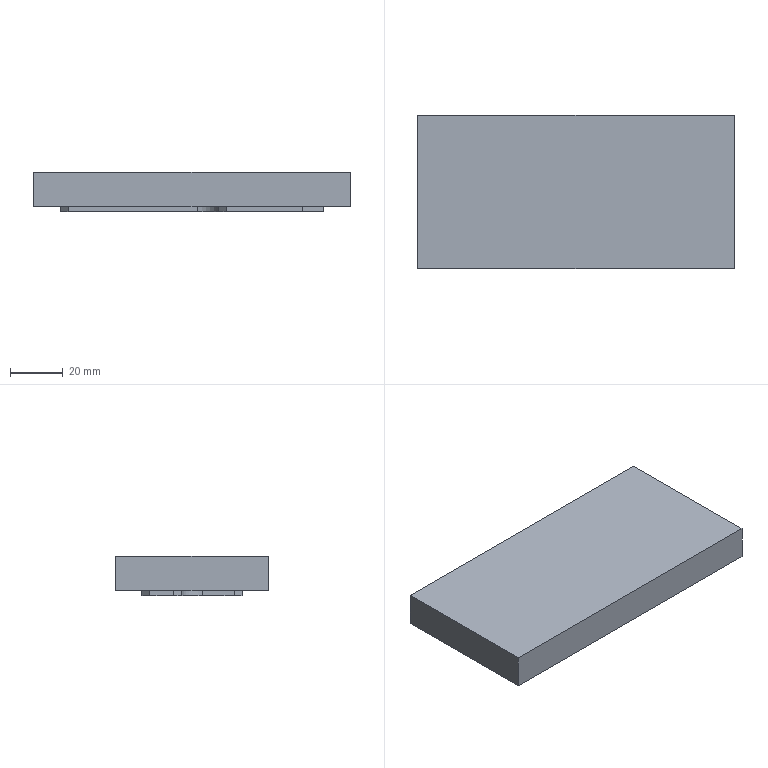Part | NX | 2 solids | 38 faces | box 120 x 58 x 15 mm | volume 90459 mm3 | plane 28 | cylinder 10 | commonest cylinder face diameters 3.4 x2 3.5 x2 4.5 x2 16 x2 24.5 x1 31.5 x1
STEP:
#1=CARTESIAN_POINT('',(30.,1.7,-5.));
#2=VERTEX_POINT('',#1);
#3=CARTESIAN_POINT('',(30.,-1.7,-5.));
#4=VERTEX_POINT('',#3);
#5=CARTESIAN_POINT('',(30.,0.,-5.));
#6=DIRECTION('',(0.,0.,1.));
#7=DIRECTION('',(0.,-1.,0.));
#8=AXIS2_PLACEMENT_3D('',#5,#6,#7);
#9=CIRCLE('',#8,1.7);
#10=EDGE_CURVE('',#2,#4,#9,.T.);
#11=ORIENTED_EDGE('',*,*,#10,.F.);
#12=CARTESIAN_POINT('',(30.,1.7,0.));
#13=VERTEX_POINT('',#12);
#14=CARTESIAN_POINT('',(30.,1.7,0.));
#15=DIRECTION('',(0.,0.,1.));
#16=VECTOR('',#15,1000.);
#17=LINE('',#14,#16);
#18=EDGE_CURVE('',#2,#13,#17,.T.);
#19=ORIENTED_EDGE('',*,*,#18,.T.);
#20=CARTESIAN_POINT('',(30.,-1.7,0.));
#21=VERTEX_POINT('',#20);
#22=CARTESIAN_POINT('',(30.,0.,0.));
#23=DIRECTION('',(0.,0.,1.));
#24=DIRECTION('',(0.,-1.,0.));
#25=AXIS2_PLACEMENT_3D('',#22,#23,#24);
#26=CIRCLE('',#25,1.7);
#27=EDGE_CURVE('',#13,#21,#26,.T.);
#28=ORIENTED_EDGE('',*,*,#27,.T.);
#29=CARTESIAN_POINT('',(30.,-1.7,0.));
#30=DIRECTION('',(0.,0.,1.));
#31=VECTOR('',#30,1000.);
#32=LINE('',#29,#31);
#33=EDGE_CURVE('',#4,#21,#32,.T.);
#34=ORIENTED_EDGE('',*,*,#33,.F.);
#35=EDGE_LOOP('',(#11,#19,#28,#34));
#36=FACE_BOUND('',#35,.T.);
#37=CARTESIAN_POINT('',(30.,0.,0.));
#38=DIRECTION('',(0.,0.,1.));
#39=DIRECTION('',(0.,1.,0.));
#40=AXIS2_PLACEMENT_3D('',#37,#38,#39);
#41=CYLINDRICAL_SURFACE('',#40,1.7);
#42=ADVANCED_FACE('',(#36),#41,.F.);
#43=CARTESIAN_POINT('',(-44.,15.25,0.));
#44=VERTEX_POINT('',#43);
#45=CARTESIAN_POINT('',(6.,15.25,0.));
#46=VERTEX_POINT('',#45);
#47=CARTESIAN_POINT('',(50.,15.25,0.));
#48=DIRECTION('',(1.,0.,0.));
#49=VECTOR('',#48,1000.);
#50=LINE('',#47,#49);
#51=EDGE_CURVE('',#44,#46,#50,.T.);
#52=ORIENTED_EDGE('',*,*,#51,.T.);
#53=CARTESIAN_POINT('',(6.,10.75,0.));
#54=VERTEX_POINT('',#53);
#55=CARTESIAN_POINT('',(6.,13.,0.));
#56=DIRECTION('',(0.,0.,-1.));
#57=DIRECTION('',(0.,1.,0.));
#58=AXIS2_PLACEMENT_3D('',#55,#56,#57);
#59=CIRCLE('',#58,2.25);
#60=EDGE_CURVE('',#46,#54,#59,.T.);
#61=ORIENTED_EDGE('',*,*,#60,.T.);
#62=CARTESIAN_POINT('',(-44.,10.75,0.));
#63=VERTEX_POINT('',#62);
#64=CARTESIAN_POINT('',(50.,10.75,0.));
#65=DIRECTION('',(-1.,0.,0.));
#66=VECTOR('',#65,1000.);
#67=LINE('',#64,#66);
#68=EDGE_CURVE('',#54,#63,#67,.T.);
#69=ORIENTED_EDGE('',*,*,#68,.T.);
#70=CARTESIAN_POINT('',(-44.,13.,0.));
#71=DIRECTION('',(0.,0.,-1.));
#72=DIRECTION('',(0.,1.,0.));
#73=AXIS2_PLACEMENT_3D('',#70,#71,#72);
#74=CIRCLE('',#73,2.25);
#75=EDGE_CURVE('',#63,#44,#74,.T.);
#76=ORIENTED_EDGE('',*,*,#75,.T.);
#77=EDGE_LOOP('',(#52,#61,#69,#76));
#78=FACE_BOUND('',#77,.T.);
#79=CARTESIAN_POINT('',(30.,-15.75,0.));
#80=VERTEX_POINT('',#79);
#81=CARTESIAN_POINT('',(30.,15.75,0.));
#82=VERTEX_POINT('',#81);
#83=CARTESIAN_POINT('',(30.,0.,0.));
#84=DIRECTION('',(0.,0.,1.));
#85=DIRECTION('',(0.,-1.,0.));
#86=AXIS2_PLACEMENT_3D('',#83,#84,#85);
#87=CIRCLE('',#86,15.75);
#88=EDGE_CURVE('',#80,#82,#87,.T.);
#89=ORIENTED_EDGE('',*,*,#88,.F.);
#90=CARTESIAN_POINT('',(30.,-12.25,0.));
#91=VERTEX_POINT('',#90);
#92=CARTESIAN_POINT('',(30.,-14.,0.));
#93=DIRECTION('',(0.,0.,1.));
#94=DIRECTION('',(0.,-1.,0.));
#95=AXIS2_PLACEMENT_3D('',#92,#93,#94);
#96=CIRCLE('',#95,1.75);
#97=EDGE_CURVE('',#91,#80,#96,.T.);
#98=ORIENTED_EDGE('',*,*,#97,.F.);
#99=CARTESIAN_POINT('',(30.,12.25,0.));
#100=VERTEX_POINT('',#99);
#101=CARTESIAN_POINT('',(30.,0.,0.));
#102=DIRECTION('',(0.,0.,-1.));
#103=DIRECTION('',(0.,-1.,0.));
#104=AXIS2_PLACEMENT_3D('',#101,#102,#103);
#105=CIRCLE('',#104,12.25);
#106=EDGE_CURVE('',#100,#91,#105,.T.);
#107=ORIENTED_EDGE('',*,*,#106,.F.);
#108=CARTESIAN_POINT('',(30.,14.,0.));
#109=DIRECTION('',(0.,0.,1.));
#110=DIRECTION('',(0.,-1.,0.));
#111=AXIS2_PLACEMENT_3D('',#108,#109,#110);
#112=CIRCLE('',#111,1.75);
#113=EDGE_CURVE('',#82,#100,#112,.T.);
#114=ORIENTED_EDGE('',*,*,#113,.F.);
#115=EDGE_LOOP('',(#89,#98,#107,#114));
#116=FACE_BOUND('',#115,.T.);
#117=CARTESIAN_POINT('',(30.,0.,0.));
#118=DIRECTION('',(0.,0.,1.));
#119=DIRECTION('',(0.,-1.,0.));
#120=AXIS2_PLACEMENT_3D('',#117,#118,#119);
#121=CIRCLE('',#120,1.7);
#122=EDGE_CURVE('',#21,#13,#121,.T.);
#123=ORIENTED_EDGE('',*,*,#122,.F.);
#124=ORIENTED_EDGE('',*,*,#27,.F.);
#125=EDGE_LOOP('',(#123,#124));
#126=FACE_BOUND('',#125,.T.);
#127=CARTESIAN_POINT('',(-50.,16.,0.));
#128=VERTEX_POINT('',#127);
#129=CARTESIAN_POINT('',(-50.,7.,0.));
#130=VERTEX_POINT('',#129);
#131=CARTESIAN_POINT('',(-50.,-19.,0.));
#132=DIRECTION('',(0.,-1.,0.));
#133=VECTOR('',#132,1000.);
#134=LINE('',#131,#133);
#135=EDGE_CURVE('',#128,#130,#134,.T.);
#136=ORIENTED_EDGE('',*,*,#135,.T.);
#137=CARTESIAN_POINT('',(-47.,4.,0.));
#138=VERTEX_POINT('',#137);
#139=CARTESIAN_POINT('',(-47.,4.,0.));
#140=DIRECTION('',(0.7071,-0.7071,0.));
#141=VECTOR('',#140,1000.);
#142=LINE('',#139,#141);
#143=EDGE_CURVE('',#130,#138,#142,.T.);
#144=ORIENTED_EDGE('',*,*,#143,.T.);
#145=CARTESIAN_POINT('',(2.,4.,0.));
#146=VERTEX_POINT('',#145);
#147=CARTESIAN_POINT('',(2.,4.,0.));
#148=DIRECTION('',(1.,0.,0.));
#149=VECTOR('',#148,1000.);
#150=LINE('',#147,#149);
#151=EDGE_CURVE('',#138,#146,#150,.T.);
#152=ORIENTED_EDGE('',*,*,#151,.T.);
#153=CARTESIAN_POINT('',(10.,-4.,0.));
#154=VERTEX_POINT('',#153);
#155=CARTESIAN_POINT('',(2.,-4.,0.));
#156=DIRECTION('',(0.,0.,-1.));
#157=DIRECTION('',(0.,1.,0.));
#158=AXIS2_PLACEMENT_3D('',#155,#156,#157);
#159=CIRCLE('',#158,8.);
#160=EDGE_CURVE('',#146,#154,#159,.T.);
#161=ORIENTED_EDGE('',*,*,#160,.T.);
#162=CARTESIAN_POINT('',(10.,-16.,0.));
#163=VERTEX_POINT('',#162);
#164=CARTESIAN_POINT('',(10.,-19.,0.));
#165=DIRECTION('',(0.,-1.,0.));
#166=VECTOR('',#165,1000.);
#167=LINE('',#164,#166);
#168=EDGE_CURVE('',#154,#163,#167,.T.);
#169=ORIENTED_EDGE('',*,*,#168,.T.);
#170=CARTESIAN_POINT('',(13.,-19.,0.));
#171=VERTEX_POINT('',#170);
#172=CARTESIAN_POINT('',(13.,-19.,0.));
#173=DIRECTION('',(0.7071,-0.7071,0.));
#174=VECTOR('',#173,1000.);
#175=LINE('',#172,#174);
#176=EDGE_CURVE('',#163,#171,#175,.T.);
#177=ORIENTED_EDGE('',*,*,#176,.T.);
#178=CARTESIAN_POINT('',(42.,-19.,0.));
#179=VERTEX_POINT('',#178);
#180=CARTESIAN_POINT('',(50.,-19.,0.));
#181=DIRECTION('',(-1.,0.,0.));
#182=VECTOR('',#181,1000.);
#183=LINE('',#180,#182);
#184=EDGE_CURVE('',#179,#171,#183,.T.);
#185=ORIENTED_EDGE('',*,*,#184,.F.);
#186=CARTESIAN_POINT('',(50.,-11.,0.));
#187=VERTEX_POINT('',#186);
#188=CARTESIAN_POINT('',(50.,-11.,0.));
#189=DIRECTION('',(0.7071,0.7071,0.));
#190=VECTOR('',#189,1000.);
#191=LINE('',#188,#190);
#192=EDGE_CURVE('',#179,#187,#191,.T.);
#193=ORIENTED_EDGE('',*,*,#192,.T.);
#194=CARTESIAN_POINT('',(50.,11.,0.));
#195=VERTEX_POINT('',#194);
#196=CARTESIAN_POINT('',(50.,-19.,0.));
#197=DIRECTION('',(0.,-1.,0.));
#198=VECTOR('',#197,1000.);
#199=LINE('',#196,#198);
#200=EDGE_CURVE('',#195,#187,#199,.T.);
#201=ORIENTED_EDGE('',*,*,#200,.F.);
#202=CARTESIAN_POINT('',(42.,19.,0.));
#203=VERTEX_POINT('',#202);
#204=CARTESIAN_POINT('',(50.,11.,0.));
#205=DIRECTION('',(-0.7071,0.7071,0.));
#206=VECTOR('',#205,1000.);
#207=LINE('',#204,#206);
#208=EDGE_CURVE('',#195,#203,#207,.T.);
#209=ORIENTED_EDGE('',*,*,#208,.T.);
#210=CARTESIAN_POINT('',(-47.,19.,0.));
#211=VERTEX_POINT('',#210);
#212=CARTESIAN_POINT('',(50.,19.,0.));
#213=DIRECTION('',(-1.,0.,0.));
#214=VECTOR('',#213,1000.);
#215=LINE('',#212,#214);
#216=EDGE_CURVE('',#203,#211,#215,.T.);
#217=ORIENTED_EDGE('',*,*,#216,.T.);
#218=CARTESIAN_POINT('',(-47.,19.,0.));
#219=DIRECTION('',(-0.7071,-0.7071,0.));
#220=VECTOR('',#219,1000.);
#221=LINE('',#218,#220);
#222=EDGE_CURVE('',#211,#128,#221,.T.);
#223=ORIENTED_EDGE('',*,*,#222,.T.);
#224=EDGE_LOOP('',(#136,#144,#152,#161,#169,#177,#185,#193,#201,#209,#217,#223));
#225=FACE_BOUND('',#224,.T.);
#226=CARTESIAN_POINT('',(50.,-19.,0.));
#227=DIRECTION('',(0.,0.,-1.));
#228=DIRECTION('',(0.,-1.,0.));
#229=AXIS2_PLACEMENT_3D('',#226,#227,#228);
#230=PLANE('',#229);
#231=ADVANCED_FACE('',(#78,#116,#126,#225),#230,.F.);
#232=ORIENTED_EDGE('',*,*,#184,.T.);
#233=CARTESIAN_POINT('',(13.,-19.,-5.));
#234=VERTEX_POINT('',#233);
#235=CARTESIAN_POINT('',(13.,-19.,-5.));
#236=DIRECTION('',(0.,0.,-1.));
#237=VECTOR('',#236,1000.);
#238=LINE('',#235,#237);
#239=EDGE_CURVE('',#171,#234,#238,.T.);
#240=ORIENTED_EDGE('',*,*,#239,.T.);
#241=CARTESIAN_POINT('',(42.,-19.,-5.));
#242=VERTEX_POINT('',#241);
#243=CARTESIAN_POINT('',(50.,-19.,-5.));
#244=DIRECTION('',(-1.,0.,0.));
#245=VECTOR('',#244,1000.);
#246=LINE('',#243,#245);
#247=EDGE_CURVE('',#242,#234,#246,.T.);
#248=ORIENTED_EDGE('',*,*,#247,.F.);
#249=CARTESIAN_POINT('',(42.,-19.,0.));
#250=DIRECTION('',(0.,0.,1.));
#251=VECTOR('',#250,1000.);
#252=LINE('',#249,#251);
#253=EDGE_CURVE('',#242,#179,#252,.T.);
#254=ORIENTED_EDGE('',*,*,#253,.T.);
#255=EDGE_LOOP('',(#232,#240,#248,#254));
#256=FACE_BOUND('',#255,.T.);
#257=CARTESIAN_POINT('',(50.,-19.,-5.));
#258=DIRECTION('',(0.,1.,0.));
#259=DIRECTION('',(0.,0.,-1.));
#260=AXIS2_PLACEMENT_3D('',#257,#258,#259);
#261=PLANE('',#260);
#262=ADVANCED_FACE('',(#256),#261,.F.);
#263=CARTESIAN_POINT('',(6.,10.75,-5.));
#264=VERTEX_POINT('',#263);
#265=CARTESIAN_POINT('',(-44.,10.75,-5.));
#266=VERTEX_POINT('',#265);
#267=CARTESIAN_POINT('',(6.,10.75,-5.));
#268=DIRECTION('',(-1.,0.,0.));
#269=VECTOR('',#268,1000.);
#270=LINE('',#267,#269);
#271=EDGE_CURVE('',#264,#266,#270,.T.);
#272=ORIENTED_EDGE('',*,*,#271,.F.);
#273=CARTESIAN_POINT('',(6.,15.25,-5.));
#274=VERTEX_POINT('',#273);
#275=CARTESIAN_POINT('',(6.,13.,-5.));
#276=DIRECTION('',(0.,0.,-1.));
#277=DIRECTION('',(0.,1.,0.));
#278=AXIS2_PLACEMENT_3D('',#275,#276,#277);
#279=CIRCLE('',#278,2.25);
#280=EDGE_CURVE('',#274,#264,#279,.T.);
#281=ORIENTED_EDGE('',*,*,#280,.F.);
#282=CARTESIAN_POINT('',(-44.,15.25,-5.));
#283=VERTEX_POINT('',#282);
#284=CARTESIAN_POINT('',(6.,15.25,-5.));
#285=DIRECTION('',(1.,0.,0.));
#286=VECTOR('',#285,1000.);
#287=LINE('',#284,#286);
#288=EDGE_CURVE('',#283,#274,#287,.T.);
#289=ORIENTED_EDGE('',*,*,#288,.F.);
#290=CARTESIAN_POINT('',(-44.,13.,-5.));
#291=DIRECTION('',(0.,0.,-1.));
#292=DIRECTION('',(0.,1.,0.));
#293=AXIS2_PLACEMENT_3D('',#290,#291,#292);
#294=CIRCLE('',#293,2.25);
#295=EDGE_CURVE('',#266,#283,#294,.T.);
#296=ORIENTED_EDGE('',*,*,#295,.F.);
#297=EDGE_LOOP('',(#272,#281,#289,#296));
#298=FACE_BOUND('',#297,.T.);
#299=CARTESIAN_POINT('',(30.,12.25,-5.));
#300=VERTEX_POINT('',#299);
#301=CARTESIAN_POINT('',(30.,-12.25,-5.));
#302=VERTEX_POINT('',#301);
#303=CARTESIAN_POINT('',(30.,0.,-5.));
#304=DIRECTION('',(0.,0.,-1.));
#305=DIRECTION('',(0.,-1.,0.));
#306=AXIS2_PLACEMENT_3D('',#303,#304,#305);
#307=CIRCLE('',#306,12.25);
#308=EDGE_CURVE('',#300,#302,#307,.T.);
#309=ORIENTED_EDGE('',*,*,#308,.T.);
#310=CARTESIAN_POINT('',(30.,-15.75,-5.));
#311=VERTEX_POINT('',#310);
#312=CARTESIAN_POINT('',(30.,-14.,-5.));
#313=DIRECTION('',(0.,0.,1.));
#314=DIRECTION('',(0.,-1.,0.));
#315=AXIS2_PLACEMENT_3D('',#312,#313,#314);
#316=CIRCLE('',#315,1.75);
#317=EDGE_CURVE('',#302,#311,#316,.T.);
#318=ORIENTED_EDGE('',*,*,#317,.T.);
#319=CARTESIAN_POINT('',(30.,15.75,-5.));
#320=VERTEX_POINT('',#319);
#321=CARTESIAN_POINT('',(30.,0.,-5.));
#322=DIRECTION('',(0.,0.,1.));
#323=DIRECTION('',(0.,-1.,0.));
#324=AXIS2_PLACEMENT_3D('',#321,#322,#323);
#325=CIRCLE('',#324,15.75);
#326=EDGE_CURVE('',#311,#320,#325,.T.);
#327=ORIENTED_EDGE('',*,*,#326,.T.);
#328=CARTESIAN_POINT('',(30.,14.,-5.));
#329=DIRECTION('',(0.,0.,1.));
#330=DIRECTION('',(0.,-1.,0.));
#331=AXIS2_PLACEMENT_3D('',#328,#329,#330);
#332=CIRCLE('',#331,1.75);
#333=EDGE_CURVE('',#320,#300,#332,.T.);
#334=ORIENTED_EDGE('',*,*,#333,.T.);
#335=EDGE_LOOP('',(#309,#318,#327,#334));
#336=FACE_BOUND('',#335,.T.);
#337=CARTESIAN_POINT('',(30.,0.,-5.));
#338=DIRECTION('',(0.,0.,1.));
#339=DIRECTION('',(0.,-1.,0.));
#340=AXIS2_PLACEMENT_3D('',#337,#338,#339);
#341=CIRCLE('',#340,1.7);
#342=EDGE_CURVE('',#4,#2,#341,.T.);
#343=ORIENTED_EDGE('',*,*,#342,.T.);
#344=ORIENTED_EDGE('',*,*,#10,.T.);
#345=EDGE_LOOP('',(#343,#344));
#346=FACE_BOUND('',#345,.T.);
#347=CARTESIAN_POINT('',(-47.,4.,-5.));
#348=VERTEX_POINT('',#347);
#349=CARTESIAN_POINT('',(2.,4.,-5.));
#350=VERTEX_POINT('',#349);
#351=CARTESIAN_POINT('',(2.,4.,-5.));
#352=DIRECTION('',(1.,0.,0.));
#353=VECTOR('',#352,1000.);
#354=LINE('',#351,#353);
#355=EDGE_CURVE('',#348,#350,#354,.T.);
#356=ORIENTED_EDGE('',*,*,#355,.F.);
#357=CARTESIAN_POINT('',(-50.,7.,-5.));
#358=VERTEX_POINT('',#357);
#359=CARTESIAN_POINT('',(-47.,4.,-5.));
#360=DIRECTION('',(-0.7071,0.7071,0.));
#361=VECTOR('',#360,1000.);
#362=LINE('',#359,#361);
#363=EDGE_CURVE('',#348,#358,#362,.T.);
#364=ORIENTED_EDGE('',*,*,#363,.T.);
#365=CARTESIAN_POINT('',(-50.,16.,-5.));
#366=VERTEX_POINT('',#365);
#367=CARTESIAN_POINT('',(-50.,-19.,-5.));
#368=DIRECTION('',(0.,1.,0.));
#369=VECTOR('',#368,1000.);
#370=LINE('',#367,#369);
#371=EDGE_CURVE('',#358,#366,#370,.T.);
#372=ORIENTED_EDGE('',*,*,#371,.T.);
#373=CARTESIAN_POINT('',(-47.,19.,-5.));
#374=VERTEX_POINT('',#373);
#375=CARTESIAN_POINT('',(-47.,19.,-5.));
#376=DIRECTION('',(0.7071,0.7071,0.));
#377=VECTOR('',#376,1000.);
#378=LINE('',#375,#377);
#379=EDGE_CURVE('',#366,#374,#378,.T.);
#380=ORIENTED_EDGE('',*,*,#379,.T.);
#381=CARTESIAN_POINT('',(42.,19.,-5.));
#382=VERTEX_POINT('',#381);
#383=CARTESIAN_POINT('',(50.,19.,-5.));
#384=DIRECTION('',(-1.,0.,0.));
#385=VECTOR('',#384,1000.);
#386=LINE('',#383,#385);
#387=EDGE_CURVE('',#382,#374,#386,.T.);
#388=ORIENTED_EDGE('',*,*,#387,.F.);
#389=CARTESIAN_POINT('',(50.,11.,-5.));
#390=VERTEX_POINT('',#389);
#391=CARTESIAN_POINT('',(50.,11.,-5.));
#392=DIRECTION('',(0.7071,-0.7071,0.));
#393=VECTOR('',#392,1000.);
#394=LINE('',#391,#393);
#395=EDGE_CURVE('',#382,#390,#394,.T.);
#396=ORIENTED_EDGE('',*,*,#395,.T.);
#397=CARTESIAN_POINT('',(50.,-11.,-5.));
#398=VERTEX_POINT('',#397);
#399=CARTESIAN_POINT('',(50.,-19.,-5.));
#400=DIRECTION('',(0.,1.,0.));
#401=VECTOR('',#400,1000.);
#402=LINE('',#399,#401);
#403=EDGE_CURVE('',#398,#390,#402,.T.);
#404=ORIENTED_EDGE('',*,*,#403,.F.);
#405=CARTESIAN_POINT('',(50.,-11.,-5.));
#406=DIRECTION('',(-0.7071,-0.7071,0.));
#407=VECTOR('',#406,1000.);
#408=LINE('',#405,#407);
#409=EDGE_CURVE('',#398,#242,#408,.T.);
#410=ORIENTED_EDGE('',*,*,#409,.T.);
#411=ORIENTED_EDGE('',*,*,#247,.T.);
#412=CARTESIAN_POINT('',(10.,-16.,-5.));
#413=VERTEX_POINT('',#412);
#414=CARTESIAN_POINT('',(13.,-19.,-5.));
#415=DIRECTION('',(-0.7071,0.7071,0.));
#416=VECTOR('',#415,1000.);
#417=LINE('',#414,#416);
#418=EDGE_CURVE('',#234,#413,#417,.T.);
#419=ORIENTED_EDGE('',*,*,#418,.T.);
#420=CARTESIAN_POINT('',(10.,-4.,-5.));
#421=VERTEX_POINT('',#420);
#422=CARTESIAN_POINT('',(10.,-19.,-5.));
#423=DIRECTION('',(0.,-1.,0.));
#424=VECTOR('',#423,1000.);
#425=LINE('',#422,#424);
#426=EDGE_CURVE('',#421,#413,#425,.T.);
#427=ORIENTED_EDGE('',*,*,#426,.F.);
#428=CARTESIAN_POINT('',(2.,-4.,-5.));
#429=DIRECTION('',(0.,0.,-1.));
#430=DIRECTION('',(0.,1.,0.));
#431=AXIS2_PLACEMENT_3D('',#428,#429,#430);
#432=CIRCLE('',#431,8.);
#433=EDGE_CURVE('',#350,#421,#432,.T.);
#434=ORIENTED_EDGE('',*,*,#433,.F.);
#435=EDGE_LOOP('',(#356,#364,#372,#380,#388,#396,#404,#410,#411,#419,#427,#434));
#436=FACE_BOUND('',#435,.T.);
#437=CARTESIAN_POINT('',(50.,-19.,-5.));
#438=DIRECTION('',(0.,0.,1.));
#439=DIRECTION('',(0.,1.,0.));
#440=AXIS2_PLACEMENT_3D('',#437,#438,#439);
#441=PLANE('',#440);
#442=ADVANCED_FACE('',(#298,#336,#346,#436),#441,.F.);
#443=ORIENTED_EDGE('',*,*,#387,.T.);
#444=CARTESIAN_POINT('',(-47.,19.,-5.));
#445=DIRECTION('',(0.,0.,1.));
#446=VECTOR('',#445,1000.);
#447=LINE('',#444,#446);
#448=EDGE_CURVE('',#374,#211,#447,.T.);
#449=ORIENTED_EDGE('',*,*,#448,.T.);
#450=ORIENTED_EDGE('',*,*,#216,.F.);
#451=CARTESIAN_POINT('',(42.,19.,-5.));
#452=DIRECTION('',(0.,0.,-1.));
#453=VECTOR('',#452,1000.);
#454=LINE('',#451,#453);
#455=EDGE_CURVE('',#203,#382,#454,.T.);
#456=ORIENTED_EDGE('',*,*,#455,.T.);
#457=EDGE_LOOP('',(#443,#449,#450,#456));
#458=FACE_BOUND('',#457,.T.);
#459=CARTESIAN_POINT('',(50.,19.,-5.));
#460=DIRECTION('',(0.,-1.,0.));
#461=DIRECTION('',(0.,0.,1.));
#462=AXIS2_PLACEMENT_3D('',#459,#460,#461);
#463=PLANE('',#462);
#464=ADVANCED_FACE('',(#458),#463,.F.);
#465=ORIENTED_EDGE('',*,*,#403,.T.);
#466=CARTESIAN_POINT('',(50.,11.,0.));
#467=DIRECTION('',(0.,0.,1.));
#468=VECTOR('',#467,1000.);
#469=LINE('',#466,#468);
#470=EDGE_CURVE('',#390,#195,#469,.T.);
#471=ORIENTED_EDGE('',*,*,#470,.T.);
#472=ORIENTED_EDGE('',*,*,#200,.T.);
#473=CARTESIAN_POINT('',(50.,-11.,-5.));
#474=DIRECTION('',(0.,0.,-1.));
#475=VECTOR('',#474,1000.);
#476=LINE('',#473,#475);
#477=EDGE_CURVE('',#187,#398,#476,.T.);
#478=ORIENTED_EDGE('',*,*,#477,.T.);
#479=EDGE_LOOP('',(#465,#471,#472,#478));
#480=FACE_BOUND('',#479,.T.);
#481=CARTESIAN_POINT('',(50.,0.,-2.5));
#482=DIRECTION('',(1.,0.,0.));
#483=DIRECTION('',(0.,-1.,0.));
#484=AXIS2_PLACEMENT_3D('',#481,#482,#483);
#485=PLANE('',#484);
#486=ADVANCED_FACE('',(#480),#485,.T.);
#487=ORIENTED_EDGE('',*,*,#371,.F.);
#488=CARTESIAN_POINT('',(-50.,7.,-2.5));
#489=DIRECTION('',(0.,0.,1.));
#490=VECTOR('',#489,1000.);
#491=LINE('',#488,#490);
#492=EDGE_CURVE('',#358,#130,#491,.T.);
#493=ORIENTED_EDGE('',*,*,#492,.T.);
#494=ORIENTED_EDGE('',*,*,#135,.F.);
#495=CARTESIAN_POINT('',(-50.,16.,-2.5));
#496=DIRECTION('',(0.,0.,-1.));
#497=VECTOR('',#496,1000.);
#498=LINE('',#495,#497);
#499=EDGE_CURVE('',#128,#366,#498,.T.);
#500=ORIENTED_EDGE('',*,*,#499,.T.);
#501=EDGE_LOOP('',(#487,#493,#494,#500));
#502=FACE_BOUND('',#501,.T.);
#503=CARTESIAN_POINT('',(-50.,0.,-2.5));
#504=DIRECTION('',(1.,0.,0.));
#505=DIRECTION('',(0.,-1.,0.));
#506=AXIS2_PLACEMENT_3D('',#503,#504,#505);
#507=PLANE('',#506);
#508=ADVANCED_FACE('',(#502),#507,.F.);
#509=ORIENTED_EDGE('',*,*,#18,.F.);
#510=ORIENTED_EDGE('',*,*,#342,.F.);
#511=ORIENTED_EDGE('',*,*,#33,.T.);
#512=ORIENTED_EDGE('',*,*,#122,.T.);
#513=EDGE_LOOP('',(#509,#510,#511,#512));
#514=FACE_BOUND('',#513,.T.);
#515=CARTESIAN_POINT('',(30.,0.,0.));
#516=DIRECTION('',(0.,0.,1.));
#517=DIRECTION('',(0.,1.,0.));
#518=AXIS2_PLACEMENT_3D('',#515,#516,#517);
#519=CYLINDRICAL_SURFACE('',#518,1.7);
#520=ADVANCED_FACE('',(#514),#519,.F.);
#521=ORIENTED_EDGE('',*,*,#97,.T.);
#522=CARTESIAN_POINT('',(30.,-15.75,-5.));
#523=DIRECTION('',(0.,0.,1.));
#524=VECTOR('',#523,1000.);
#525=LINE('',#522,#524);
#526=EDGE_CURVE('',#311,#80,#525,.T.);
#527=ORIENTED_EDGE('',*,*,#526,.F.);
#528=ORIENTED_EDGE('',*,*,#317,.F.);
#529=CARTESIAN_POINT('',(30.,-12.25,-5.));
#530=DIRECTION('',(0.,0.,1.));
#531=VECTOR('',#530,1000.);
#532=LINE('',#529,#531);
#533=EDGE_CURVE('',#302,#91,#532,.T.);
#534=ORIENTED_EDGE('',*,*,#533,.T.);
#535=EDGE_LOOP('',(#521,#527,#528,#534));
#536=FACE_BOUND('',#535,.T.);
#537=CARTESIAN_POINT('',(30.,-14.,-5.));
#538=DIRECTION('',(0.,0.,1.));
#539=DIRECTION('',(0.,1.,0.));
#540=AXIS2_PLACEMENT_3D('',#537,#538,#539);
#541=CYLINDRICAL_SURFACE('',#540,1.75);
#542=ADVANCED_FACE('',(#536),#541,.F.);
#543=ORIENTED_EDGE('',*,*,#106,.T.);
#544=ORIENTED_EDGE('',*,*,#533,.F.);
#545=ORIENTED_EDGE('',*,*,#308,.F.);
#546=CARTESIAN_POINT('',(30.,12.25,-5.));
#547=DIRECTION('',(0.,0.,1.));
#548=VECTOR('',#547,1000.);
#549=LINE('',#546,#548);
#550=EDGE_CURVE('',#300,#100,#549,.T.);
#551=ORIENTED_EDGE('',*,*,#550,.T.);
#552=EDGE_LOOP('',(#543,#544,#545,#551));
#553=FACE_BOUND('',#552,.T.);
#554=CARTESIAN_POINT('',(30.,0.,-5.));
#555=DIRECTION('',(0.,0.,1.));
#556=DIRECTION('',(0.,1.,0.));
#557=AXIS2_PLACEMENT_3D('',#554,#555,#556);
#558=CYLINDRICAL_SURFACE('',#557,12.25);
#559=ADVANCED_FACE('',(#553),#558,.T.);
#560=ORIENTED_EDGE('',*,*,#113,.T.);
#561=ORIENTED_EDGE('',*,*,#550,.F.);
#562=ORIENTED_EDGE('',*,*,#333,.F.);
#563=CARTESIAN_POINT('',(30.,15.75,-5.));
#564=DIRECTION('',(0.,0.,1.));
#565=VECTOR('',#564,1000.);
#566=LINE('',#563,#565);
#567=EDGE_CURVE('',#320,#82,#566,.T.);
#568=ORIENTED_EDGE('',*,*,#567,.T.);
#569=EDGE_LOOP('',(#560,#561,#562,#568));
#570=FACE_BOUND('',#569,.T.);
#571=CARTESIAN_POINT('',(30.,14.,-5.));
#572=DIRECTION('',(0.,0.,1.));
#573=DIRECTION('',(0.,1.,0.));
#574=AXIS2_PLACEMENT_3D('',#571,#572,#573);
#575=CYLINDRICAL_SURFACE('',#574,1.75);
#576=ADVANCED_FACE('',(#570),#575,.F.);
#577=ORIENTED_EDGE('',*,*,#88,.T.);
#578=ORIENTED_EDGE('',*,*,#567,.F.);
#579=ORIENTED_EDGE('',*,*,#326,.F.);
#580=ORIENTED_EDGE('',*,*,#526,.T.);
#581=EDGE_LOOP('',(#577,#578,#579,#580));
#582=FACE_BOUND('',#581,.T.);
#583=CARTESIAN_POINT('',(30.,0.,-5.));
#584=DIRECTION('',(0.,0.,1.));
#585=DIRECTION('',(0.,1.,0.));
#586=AXIS2_PLACEMENT_3D('',#583,#584,#585);
#587=CYLINDRICAL_SURFACE('',#586,15.75);
#588=ADVANCED_FACE('',(#582),#587,.F.);
#589=CARTESIAN_POINT('',(6.,15.25,5.));
#590=DIRECTION('',(0.,0.,-1.));
#591=VECTOR('',#590,1000.);
#592=LINE('',#589,#591);
#593=EDGE_CURVE('',#46,#274,#592,.T.);
#594=ORIENTED_EDGE('',*,*,#593,.T.);
#595=ORIENTED_EDGE('',*,*,#280,.T.);
#596=CARTESIAN_POINT('',(6.,10.75,5.));
#597=DIRECTION('',(0.,0.,-1.));
#598=VECTOR('',#597,1000.);
#599=LINE('',#596,#598);
#600=EDGE_CURVE('',#54,#264,#599,.T.);
#601=ORIENTED_EDGE('',*,*,#600,.F.);
#602=ORIENTED_EDGE('',*,*,#60,.F.);
#603=EDGE_LOOP('',(#594,#595,#601,#602));
#604=FACE_BOUND('',#603,.T.);
#605=CARTESIAN_POINT('',(6.,13.,5.));
#606=DIRECTION('',(0.,0.,-1.));
#607=DIRECTION('',(0.,-1.,0.));
#608=AXIS2_PLACEMENT_3D('',#605,#606,#607);
#609=CYLINDRICAL_SURFACE('',#608,2.25);
#610=ADVANCED_FACE('',(#604),#609,.F.);
#611=CARTESIAN_POINT('',(-44.,15.25,5.));
#612=DIRECTION('',(0.,0.,-1.));
#613=VECTOR('',#612,1000.);
#614=LINE('',#611,#613);
#615=EDGE_CURVE('',#44,#283,#614,.T.);
#616=ORIENTED_EDGE('',*,*,#615,.T.);
#617=ORIENTED_EDGE('',*,*,#288,.T.);
#618=ORIENTED_EDGE('',*,*,#593,.F.);
#619=ORIENTED_EDGE('',*,*,#51,.F.);
#620=EDGE_LOOP('',(#616,#617,#618,#619));
#621=FACE_BOUND('',#620,.T.);
#622=CARTESIAN_POINT('',(6.,15.25,5.));
#623=DIRECTION('',(0.,1.,0.));
#624=DIRECTION('',(0.,0.,-1.));
#625=AXIS2_PLACEMENT_3D('',#622,#623,#624);
#626=PLANE('',#625);
#627=ADVANCED_FACE('',(#621),#626,.F.);
#628=CARTESIAN_POINT('',(-44.,10.75,5.));
#629=DIRECTION('',(0.,0.,-1.));
#630=VECTOR('',#629,1000.);
#631=LINE('',#628,#630);
#632=EDGE_CURVE('',#63,#266,#631,.T.);
#633=ORIENTED_EDGE('',*,*,#632,.T.);
#634=ORIENTED_EDGE('',*,*,#295,.T.);
#635=ORIENTED_EDGE('',*,*,#615,.F.);
#636=ORIENTED_EDGE('',*,*,#75,.F.);
#637=EDGE_LOOP('',(#633,#634,#635,#636));
#638=FACE_BOUND('',#637,.T.);
#639=CARTESIAN_POINT('',(-44.,13.,5.));
#640=DIRECTION('',(0.,0.,-1.));
#641=DIRECTION('',(0.,-1.,0.));
#642=AXIS2_PLACEMENT_3D('',#639,#640,#641);
#643=CYLINDRICAL_SURFACE('',#642,2.25);
#644=ADVANCED_FACE('',(#638),#643,.F.);
#645=ORIENTED_EDGE('',*,*,#600,.T.);
#646=ORIENTED_EDGE('',*,*,#271,.T.);
#647=ORIENTED_EDGE('',*,*,#632,.F.);
#648=ORIENTED_EDGE('',*,*,#68,.F.);
#649=EDGE_LOOP('',(#645,#646,#647,#648));
#650=FACE_BOUND('',#649,.T.);
#651=CARTESIAN_POINT('',(6.,10.75,5.));
#652=DIRECTION('',(0.,-1.,0.));
#653=DIRECTION('',(0.,0.,1.));
#654=AXIS2_PLACEMENT_3D('',#651,#652,#653);
#655=PLANE('',#654);
#656=ADVANCED_FACE('',(#650),#655,.F.);
#657=ORIENTED_EDGE('',*,*,#395,.F.);
#658=ORIENTED_EDGE('',*,*,#455,.F.);
#659=ORIENTED_EDGE('',*,*,#208,.F.);
#660=ORIENTED_EDGE('',*,*,#470,.F.);
#661=EDGE_LOOP('',(#657,#658,#659,#660));
#662=FACE_BOUND('',#661,.T.);
#663=CARTESIAN_POINT('',(50.,11.,-2.5));
#664=DIRECTION('',(0.7071,0.7071,0.));
#665=DIRECTION('',(0.,0.,1.));
#666=AXIS2_PLACEMENT_3D('',#663,#664,#665);
#667=PLANE('',#666);
#668=ADVANCED_FACE('',(#662),#667,.T.);
#669=ORIENTED_EDGE('',*,*,#192,.F.);
#670=ORIENTED_EDGE('',*,*,#253,.F.);
#671=ORIENTED_EDGE('',*,*,#409,.F.);
#672=ORIENTED_EDGE('',*,*,#477,.F.);
#673=EDGE_LOOP('',(#669,#670,#671,#672));
#674=FACE_BOUND('',#673,.T.);
#675=CARTESIAN_POINT('',(50.,-11.,-2.5));
#676=DIRECTION('',(0.7071,-0.7071,0.));
#677=DIRECTION('',(0.,0.,-1.));
#678=AXIS2_PLACEMENT_3D('',#675,#676,#677);
#679=PLANE('',#678);
#680=ADVANCED_FACE('',(#674),#679,.T.);
#681=ORIENTED_EDGE('',*,*,#426,.T.);
#682=CARTESIAN_POINT('',(10.,-16.,0.));
#683=DIRECTION('',(0.,0.,1.));
#684=VECTOR('',#683,1000.);
#685=LINE('',#682,#684);
#686=EDGE_CURVE('',#413,#163,#685,.T.);
#687=ORIENTED_EDGE('',*,*,#686,.T.);
#688=ORIENTED_EDGE('',*,*,#168,.F.);
#689=CARTESIAN_POINT('',(10.,-4.,0.));
#690=DIRECTION('',(0.,0.,-1.));
#691=VECTOR('',#690,1000.);
#692=LINE('',#689,#691);
#693=EDGE_CURVE('',#154,#421,#692,.T.);
#694=ORIENTED_EDGE('',*,*,#693,.T.);
#695=EDGE_LOOP('',(#681,#687,#688,#694));
#696=FACE_BOUND('',#695,.T.);
#697=CARTESIAN_POINT('',(10.,-19.,0.));
#698=DIRECTION('',(1.,0.,0.));
#699=DIRECTION('',(0.,-1.,0.));
#700=AXIS2_PLACEMENT_3D('',#697,#698,#699);
#701=PLANE('',#700);
#702=ADVANCED_FACE('',(#696),#701,.F.);
#703=ORIENTED_EDGE('',*,*,#433,.T.);
#704=ORIENTED_EDGE('',*,*,#693,.F.);
#705=ORIENTED_EDGE('',*,*,#160,.F.);
#706=CARTESIAN_POINT('',(2.,4.,0.));
#707=DIRECTION('',(0.,0.,-1.));
#708=VECTOR('',#707,1000.);
#709=LINE('',#706,#708);
#710=EDGE_CURVE('',#146,#350,#709,.T.);
#711=ORIENTED_EDGE('',*,*,#710,.T.);
#712=EDGE_LOOP('',(#703,#704,#705,#711));
#713=FACE_BOUND('',#712,.T.);
#714=CARTESIAN_POINT('',(2.,-4.,0.));
#715=DIRECTION('',(0.,0.,-1.));
#716=DIRECTION('',(0.,-1.,0.));
#717=AXIS2_PLACEMENT_3D('',#714,#715,#716);
#718=CYLINDRICAL_SURFACE('',#717,8.);
#719=ADVANCED_FACE('',(#713),#718,.F.);
#720=ORIENTED_EDGE('',*,*,#151,.F.);
#721=CARTESIAN_POINT('',(-47.,4.,0.));
#722=DIRECTION('',(0.,0.,-1.));
#723=VECTOR('',#722,1000.);
#724=LINE('',#721,#723);
#725=EDGE_CURVE('',#138,#348,#724,.T.);
#726=ORIENTED_EDGE('',*,*,#725,.T.);
#727=ORIENTED_EDGE('',*,*,#355,.T.);
#728=ORIENTED_EDGE('',*,*,#710,.F.);
#729=EDGE_LOOP('',(#720,#726,#727,#728));
#730=FACE_BOUND('',#729,.T.);
#731=CARTESIAN_POINT('',(2.,4.,0.));
#732=DIRECTION('',(0.,1.,0.));
#733=DIRECTION('',(1.,0.,0.));
#734=AXIS2_PLACEMENT_3D('',#731,#732,#733);
#735=PLANE('',#734);
#736=ADVANCED_FACE('',(#730),#735,.F.);
#737=ORIENTED_EDGE('',*,*,#143,.F.);
#738=ORIENTED_EDGE('',*,*,#492,.F.);
#739=ORIENTED_EDGE('',*,*,#363,.F.);
#740=ORIENTED_EDGE('',*,*,#725,.F.);
#741=EDGE_LOOP('',(#737,#738,#739,#740));
#742=FACE_BOUND('',#741,.T.);
#743=CARTESIAN_POINT('',(-47.,4.,0.));
#744=DIRECTION('',(0.7071,0.7071,0.));
#745=DIRECTION('',(0.,0.,1.));
#746=AXIS2_PLACEMENT_3D('',#743,#744,#745);
#747=PLANE('',#746);
#748=ADVANCED_FACE('',(#742),#747,.F.);
#749=ORIENTED_EDGE('',*,*,#379,.F.);
#750=ORIENTED_EDGE('',*,*,#499,.F.);
#751=ORIENTED_EDGE('',*,*,#222,.F.);
#752=ORIENTED_EDGE('',*,*,#448,.F.);
#753=EDGE_LOOP('',(#749,#750,#751,#752));
#754=FACE_BOUND('',#753,.T.);
#755=CARTESIAN_POINT('',(-47.,19.,-5.));
#756=DIRECTION('',(0.7071,-0.7071,0.));
#757=DIRECTION('',(0.,0.,-1.));
#758=AXIS2_PLACEMENT_3D('',#755,#756,#757);
#759=PLANE('',#758);
#760=ADVANCED_FACE('',(#754),#759,.F.);
#761=ORIENTED_EDGE('',*,*,#176,.F.);
#762=ORIENTED_EDGE('',*,*,#686,.F.);
#763=ORIENTED_EDGE('',*,*,#418,.F.);
#764=ORIENTED_EDGE('',*,*,#239,.F.);
#765=EDGE_LOOP('',(#761,#762,#763,#764));
#766=FACE_BOUND('',#765,.T.);
#767=CARTESIAN_POINT('',(13.,-19.,-5.));
#768=DIRECTION('',(0.7071,0.7071,0.));
#769=DIRECTION('',(0.,0.,1.));
#770=AXIS2_PLACEMENT_3D('',#767,#768,#769);
#771=PLANE('',#770);
#772=ADVANCED_FACE('',(#766),#771,.F.);
#773=CLOSED_SHELL('',(#42,#231,#262,#442,#464,#486,#508,#520,#542,#559,#576,#588,#610,#627,#644,#656,#668,#680,#702,#719,#736,#748,#760,#772));
#774=MANIFOLD_SOLID_BREP('',#773);
#775=CARTESIAN_POINT('',(60.,-29.,-3.));
#776=VERTEX_POINT('',#775);
#777=CARTESIAN_POINT('',(60.,29.,-3.));
#778=VERTEX_POINT('',#777);
#779=CARTESIAN_POINT('',(60.,0.,-3.));
#780=DIRECTION('',(0.,-1.,0.));
#781=VECTOR('',#780,1000.);
#782=LINE('',#779,#781);
#783=EDGE_CURVE('',#776,#778,#782,.F.);
#784=ORIENTED_EDGE('',*,*,#783,.F.);
#785=CARTESIAN_POINT('',(-60.,-29.,-3.));
#786=VERTEX_POINT('',#785);
#787=CARTESIAN_POINT('',(0.,-29.,-3.));
#788=DIRECTION('',(-1.,0.,0.));
#789=VECTOR('',#788,1000.);
#790=LINE('',#787,#789);
#791=EDGE_CURVE('',#786,#776,#790,.F.);
#792=ORIENTED_EDGE('',*,*,#791,.F.);
#793=CARTESIAN_POINT('',(-60.,29.,-3.));
#794=VERTEX_POINT('',#793);
#795=CARTESIAN_POINT('',(-60.,0.,-3.));
#796=DIRECTION('',(0.,1.,0.));
#797=VECTOR('',#796,1000.);
#798=LINE('',#795,#797);
#799=EDGE_CURVE('',#794,#786,#798,.F.);
#800=ORIENTED_EDGE('',*,*,#799,.F.);
#801=CARTESIAN_POINT('',(0.,29.,-3.));
#802=DIRECTION('',(1.,0.,0.));
#803=VECTOR('',#802,1000.);
#804=LINE('',#801,#803);
#805=EDGE_CURVE('',#778,#794,#804,.F.);
#806=ORIENTED_EDGE('',*,*,#805,.F.);
#807=EDGE_LOOP('',(#784,#792,#800,#806));
#808=FACE_BOUND('',#807,.T.);
#809=CARTESIAN_POINT('',(50.,-19.,-3.));
#810=VERTEX_POINT('',#809);
#811=CARTESIAN_POINT('',(50.,19.,-3.));
#812=VERTEX_POINT('',#811);
#813=CARTESIAN_POINT('',(50.,-19.,-3.));
#814=DIRECTION('',(0.,-1.,0.));
#815=VECTOR('',#814,1000.);
#816=LINE('',#813,#815);
#817=EDGE_CURVE('',#810,#812,#816,.F.);
#818=ORIENTED_EDGE('',*,*,#817,.T.);
#819=CARTESIAN_POINT('',(-50.,19.,-3.));
#820=VERTEX_POINT('',#819);
#821=CARTESIAN_POINT('',(50.,19.,-3.));
#822=DIRECTION('',(1.,0.,0.));
#823=VECTOR('',#822,1000.);
#824=LINE('',#821,#823);
#825=EDGE_CURVE('',#812,#820,#824,.F.);
#826=ORIENTED_EDGE('',*,*,#825,.T.);
#827=CARTESIAN_POINT('',(-50.,4.,-3.));
#828=VERTEX_POINT('',#827);
#829=CARTESIAN_POINT('',(-50.,-19.,-3.));
#830=DIRECTION('',(0.,1.,0.));
#831=VECTOR('',#830,1000.);
#832=LINE('',#829,#831);
#833=EDGE_CURVE('',#820,#828,#832,.F.);
#834=ORIENTED_EDGE('',*,*,#833,.T.);
#835=CARTESIAN_POINT('',(2.,4.,-3.));
#836=VERTEX_POINT('',#835);
#837=CARTESIAN_POINT('',(50.,4.,-3.));
#838=DIRECTION('',(-1.,0.,0.));
#839=VECTOR('',#838,1000.);
#840=LINE('',#837,#839);
#841=EDGE_CURVE('',#828,#836,#840,.F.);
#842=ORIENTED_EDGE('',*,*,#841,.T.);
#843=CARTESIAN_POINT('',(10.,-4.,-3.));
#844=VERTEX_POINT('',#843);
#845=CARTESIAN_POINT('',(2.,-4.,-3.));
#846=DIRECTION('',(0.,0.,1.));
#847=DIRECTION('',(0.,-1.,0.));
#848=AXIS2_PLACEMENT_3D('',#845,#846,#847);
#849=CIRCLE('',#848,8.);
#850=EDGE_CURVE('',#836,#844,#849,.F.);
#851=ORIENTED_EDGE('',*,*,#850,.T.);
#852=CARTESIAN_POINT('',(10.,-19.,-3.));
#853=VERTEX_POINT('',#852);
#854=CARTESIAN_POINT('',(10.,-19.,-3.));
#855=DIRECTION('',(0.,1.,0.));
#856=VECTOR('',#855,1000.);
#857=LINE('',#854,#856);
#858=EDGE_CURVE('',#844,#853,#857,.F.);
#859=ORIENTED_EDGE('',*,*,#858,.T.);
#860=CARTESIAN_POINT('',(50.,-19.,-3.));
#861=DIRECTION('',(-1.,0.,0.));
#862=VECTOR('',#861,1000.);
#863=LINE('',#860,#862);
#864=EDGE_CURVE('',#853,#810,#863,.F.);
#865=ORIENTED_EDGE('',*,*,#864,.T.);
#866=EDGE_LOOP('',(#818,#826,#834,#842,#851,#859,#865));
#867=FACE_BOUND('',#866,.T.);
#868=CARTESIAN_POINT('',(50.,-19.,-3.));
#869=DIRECTION('',(0.,0.,1.));
#870=DIRECTION('',(0.,1.,0.));
#871=AXIS2_PLACEMENT_3D('',#868,#869,#870);
#872=PLANE('',#871);
#873=ADVANCED_FACE('',(#808,#867),#872,.F.);
#874=CARTESIAN_POINT('',(60.,-29.,10.));
#875=VERTEX_POINT('',#874);
#876=CARTESIAN_POINT('',(-60.,-29.,10.));
#877=VERTEX_POINT('',#876);
#878=CARTESIAN_POINT('',(0.,-29.,10.));
#879=DIRECTION('',(-1.,0.,0.));
#880=VECTOR('',#879,1000.);
#881=LINE('',#878,#880);
#882=EDGE_CURVE('',#875,#877,#881,.T.);
#883=ORIENTED_EDGE('',*,*,#882,.F.);
#884=CARTESIAN_POINT('',(60.,29.,10.));
#885=VERTEX_POINT('',#884);
#886=CARTESIAN_POINT('',(60.,0.,10.));
#887=DIRECTION('',(0.,-1.,0.));
#888=VECTOR('',#887,1000.);
#889=LINE('',#886,#888);
#890=EDGE_CURVE('',#885,#875,#889,.T.);
#891=ORIENTED_EDGE('',*,*,#890,.F.);
#892=CARTESIAN_POINT('',(-60.,29.,10.));
#893=VERTEX_POINT('',#892);
#894=CARTESIAN_POINT('',(0.,29.,10.));
#895=DIRECTION('',(1.,0.,0.));
#896=VECTOR('',#895,1000.);
#897=LINE('',#894,#896);
#898=EDGE_CURVE('',#893,#885,#897,.T.);
#899=ORIENTED_EDGE('',*,*,#898,.F.);
#900=CARTESIAN_POINT('',(-60.,0.,10.));
#901=DIRECTION('',(0.,1.,0.));
#902=VECTOR('',#901,1000.);
#903=LINE('',#900,#902);
#904=EDGE_CURVE('',#877,#893,#903,.T.);
#905=ORIENTED_EDGE('',*,*,#904,.F.);
#906=EDGE_LOOP('',(#883,#891,#899,#905));
#907=FACE_BOUND('',#906,.T.);
#908=CARTESIAN_POINT('',(0.,0.,10.));
#909=DIRECTION('',(0.,0.,1.));
#910=DIRECTION('',(1.,0.,0.));
#911=AXIS2_PLACEMENT_3D('',#908,#909,#910);
#912=PLANE('',#911);
#913=ADVANCED_FACE('',(#907),#912,.T.);
#914=CARTESIAN_POINT('',(60.,-29.,-15.));
#915=DIRECTION('',(0.,0.,1.));
#916=VECTOR('',#915,1000.);
#917=LINE('',#914,#916);
#918=EDGE_CURVE('',#776,#875,#917,.T.);
#919=ORIENTED_EDGE('',*,*,#918,.T.);
#920=ORIENTED_EDGE('',*,*,#882,.T.);
#921=CARTESIAN_POINT('',(-60.,-29.,-15.));
#922=DIRECTION('',(0.,0.,1.));
#923=VECTOR('',#922,1000.);
#924=LINE('',#921,#923);
#925=EDGE_CURVE('',#786,#877,#924,.T.);
#926=ORIENTED_EDGE('',*,*,#925,.F.);
#927=ORIENTED_EDGE('',*,*,#791,.T.);
#928=EDGE_LOOP('',(#919,#920,#926,#927));
#929=FACE_BOUND('',#928,.T.);
#930=CARTESIAN_POINT('',(0.,-29.,-15.));
#931=DIRECTION('',(0.,-1.,0.));
#932=DIRECTION('',(0.,0.,-1.));
#933=AXIS2_PLACEMENT_3D('',#930,#931,#932);
#934=PLANE('',#933);
#935=ADVANCED_FACE('',(#929),#934,.T.);
#936=ORIENTED_EDGE('',*,*,#925,.T.);
#937=ORIENTED_EDGE('',*,*,#904,.T.);
#938=CARTESIAN_POINT('',(-60.,29.,-15.));
#939=DIRECTION('',(0.,0.,1.));
#940=VECTOR('',#939,1000.);
#941=LINE('',#938,#940);
#942=EDGE_CURVE('',#794,#893,#941,.T.);
#943=ORIENTED_EDGE('',*,*,#942,.F.);
#944=ORIENTED_EDGE('',*,*,#799,.T.);
#945=EDGE_LOOP('',(#936,#937,#943,#944));
#946=FACE_BOUND('',#945,.T.);
#947=CARTESIAN_POINT('',(-60.,0.,-15.));
#948=DIRECTION('',(-1.,0.,0.));
#949=DIRECTION('',(0.,0.,1.));
#950=AXIS2_PLACEMENT_3D('',#947,#948,#949);
#951=PLANE('',#950);
#952=ADVANCED_FACE('',(#946),#951,.T.);
#953=ORIENTED_EDGE('',*,*,#942,.T.);
#954=ORIENTED_EDGE('',*,*,#898,.T.);
#955=CARTESIAN_POINT('',(60.,29.,-15.));
#956=DIRECTION('',(0.,0.,1.));
#957=VECTOR('',#956,1000.);
#958=LINE('',#955,#957);
#959=EDGE_CURVE('',#778,#885,#958,.T.);
#960=ORIENTED_EDGE('',*,*,#959,.F.);
#961=ORIENTED_EDGE('',*,*,#805,.T.);
#962=EDGE_LOOP('',(#953,#954,#960,#961));
#963=FACE_BOUND('',#962,.T.);
#964=CARTESIAN_POINT('',(0.,29.,-15.));
#965=DIRECTION('',(0.,1.,0.));
#966=DIRECTION('',(0.,0.,1.));
#967=AXIS2_PLACEMENT_3D('',#964,#965,#966);
#968=PLANE('',#967);
#969=ADVANCED_FACE('',(#963),#968,.T.);
#970=ORIENTED_EDGE('',*,*,#783,.T.);
#971=ORIENTED_EDGE('',*,*,#959,.T.);
#972=ORIENTED_EDGE('',*,*,#890,.T.);
#973=ORIENTED_EDGE('',*,*,#918,.F.);
#974=EDGE_LOOP('',(#970,#971,#972,#973));
#975=FACE_BOUND('',#974,.T.);
#976=CARTESIAN_POINT('',(60.,0.,-15.));
#977=DIRECTION('',(1.,0.,0.));
#978=DIRECTION('',(0.,0.,-1.));
#979=AXIS2_PLACEMENT_3D('',#976,#977,#978);
#980=PLANE('',#979);
#981=ADVANCED_FACE('',(#975),#980,.T.);
#982=ORIENTED_EDGE('',*,*,#825,.F.);
#983=CARTESIAN_POINT('',(50.,19.,1.));
#984=VERTEX_POINT('',#983);
#985=CARTESIAN_POINT('',(50.,19.,1.));
#986=DIRECTION('',(0.,0.,1.));
#987=VECTOR('',#986,1000.);
#988=LINE('',#985,#987);
#989=EDGE_CURVE('',#812,#984,#988,.T.);
#990=ORIENTED_EDGE('',*,*,#989,.T.);
#991=CARTESIAN_POINT('',(-50.,19.,1.));
#992=VERTEX_POINT('',#991);
#993=CARTESIAN_POINT('',(42.,19.,1.));
#994=DIRECTION('',(-1.,0.,0.));
#995=VECTOR('',#994,1000.);
#996=LINE('',#993,#995);
#997=EDGE_CURVE('',#992,#984,#996,.F.);
#998=ORIENTED_EDGE('',*,*,#997,.F.);
#999=CARTESIAN_POINT('',(-50.,19.,1.));
#1000=DIRECTION('',(0.,0.,1.));
#1001=VECTOR('',#1000,1000.);
#1002=LINE('',#999,#1001);
#1003=EDGE_CURVE('',#820,#992,#1002,.T.);
#1004=ORIENTED_EDGE('',*,*,#1003,.F.);
#1005=EDGE_LOOP('',(#982,#990,#998,#1004));
#1006=FACE_BOUND('',#1005,.T.);
#1007=CARTESIAN_POINT('',(42.,19.,1.));
#1008=DIRECTION('',(0.,-1.,0.));
#1009=DIRECTION('',(0.,0.,-1.));
#1010=AXIS2_PLACEMENT_3D('',#1007,#1008,#1009);
#1011=PLANE('',#1010);
#1012=ADVANCED_FACE('',(#1006),#1011,.T.);
#1013=ORIENTED_EDGE('',*,*,#833,.F.);
#1014=ORIENTED_EDGE('',*,*,#1003,.T.);
#1015=CARTESIAN_POINT('',(-50.,4.,1.));
#1016=VERTEX_POINT('',#1015);
#1017=CARTESIAN_POINT('',(-50.,16.,1.));
#1018=DIRECTION('',(0.,-1.,0.));
#1019=VECTOR('',#1018,1000.);
#1020=LINE('',#1017,#1019);
#1021=EDGE_CURVE('',#1016,#992,#1020,.F.);
#1022=ORIENTED_EDGE('',*,*,#1021,.F.);
#1023=CARTESIAN_POINT('',(-50.,4.,1.));
#1024=DIRECTION('',(0.,0.,1.));
#1025=VECTOR('',#1024,1000.);
#1026=LINE('',#1023,#1025);
#1027=EDGE_CURVE('',#828,#1016,#1026,.T.);
#1028=ORIENTED_EDGE('',*,*,#1027,.F.);
#1029=EDGE_LOOP('',(#1013,#1014,#1022,#1028));
#1030=FACE_BOUND('',#1029,.T.);
#1031=CARTESIAN_POINT('',(-50.,16.,1.));
#1032=DIRECTION('',(1.,0.,0.));
#1033=DIRECTION('',(0.,0.,-1.));
#1034=AXIS2_PLACEMENT_3D('',#1031,#1032,#1033);
#1035=PLANE('',#1034);
#1036=ADVANCED_FACE('',(#1030),#1035,.T.);
#1037=ORIENTED_EDGE('',*,*,#841,.F.);
#1038=ORIENTED_EDGE('',*,*,#1027,.T.);
#1039=CARTESIAN_POINT('',(2.,4.,1.));
#1040=VERTEX_POINT('',#1039);
#1041=CARTESIAN_POINT('',(-47.,4.,1.));
#1042=DIRECTION('',(1.,0.,0.));
#1043=VECTOR('',#1042,1000.);
#1044=LINE('',#1041,#1043);
#1045=EDGE_CURVE('',#1040,#1016,#1044,.F.);
#1046=ORIENTED_EDGE('',*,*,#1045,.F.);
#1047=CARTESIAN_POINT('',(2.,4.,1.));
#1048=DIRECTION('',(0.,0.,-1.));
#1049=VECTOR('',#1048,1000.);
#1050=LINE('',#1047,#1049);
#1051=EDGE_CURVE('',#836,#1040,#1050,.F.);
#1052=ORIENTED_EDGE('',*,*,#1051,.F.);
#1053=EDGE_LOOP('',(#1037,#1038,#1046,#1052));
#1054=FACE_BOUND('',#1053,.T.);
#1055=CARTESIAN_POINT('',(-47.,4.,1.));
#1056=DIRECTION('',(0.,1.,0.));
#1057=DIRECTION('',(-1.,0.,0.));
#1058=AXIS2_PLACEMENT_3D('',#1055,#1056,#1057);
#1059=PLANE('',#1058);
#1060=ADVANCED_FACE('',(#1054),#1059,.T.);
#1061=ORIENTED_EDGE('',*,*,#850,.F.);
#1062=ORIENTED_EDGE('',*,*,#1051,.T.);
#1063=CARTESIAN_POINT('',(10.,-4.,1.));
#1064=VERTEX_POINT('',#1063);
#1065=CARTESIAN_POINT('',(2.,-4.,1.));
#1066=DIRECTION('',(0.,0.,-1.));
#1067=DIRECTION('',(0.,1.,0.));
#1068=AXIS2_PLACEMENT_3D('',#1065,#1066,#1067);
#1069=CIRCLE('',#1068,8.);
#1070=EDGE_CURVE('',#1064,#1040,#1069,.F.);
#1071=ORIENTED_EDGE('',*,*,#1070,.F.);
#1072=CARTESIAN_POINT('',(10.,-4.,1.));
#1073=DIRECTION('',(0.,0.,-1.));
#1074=VECTOR('',#1073,1000.);
#1075=LINE('',#1072,#1074);
#1076=EDGE_CURVE('',#844,#1064,#1075,.F.);
#1077=ORIENTED_EDGE('',*,*,#1076,.F.);
#1078=EDGE_LOOP('',(#1061,#1062,#1071,#1077));
#1079=FACE_BOUND('',#1078,.T.);
#1080=CARTESIAN_POINT('',(2.,-4.,1.));
#1081=DIRECTION('',(0.,0.,-1.));
#1082=DIRECTION('',(-1.,0.,0.));
#1083=AXIS2_PLACEMENT_3D('',#1080,#1081,#1082);
#1084=CYLINDRICAL_SURFACE('',#1083,8.);
#1085=ADVANCED_FACE('',(#1079),#1084,.T.);
#1086=ORIENTED_EDGE('',*,*,#858,.F.);
#1087=ORIENTED_EDGE('',*,*,#1076,.T.);
#1088=CARTESIAN_POINT('',(10.,-19.,1.));
#1089=VERTEX_POINT('',#1088);
#1090=CARTESIAN_POINT('',(10.,-4.,1.));
#1091=DIRECTION('',(0.,-1.,0.));
#1092=VECTOR('',#1091,1000.);
#1093=LINE('',#1090,#1092);
#1094=EDGE_CURVE('',#1089,#1064,#1093,.F.);
#1095=ORIENTED_EDGE('',*,*,#1094,.F.);
#1096=CARTESIAN_POINT('',(10.,-19.,1.));
#1097=DIRECTION('',(0.,0.,1.));
#1098=VECTOR('',#1097,1000.);
#1099=LINE('',#1096,#1098);
#1100=EDGE_CURVE('',#853,#1089,#1099,.T.);
#1101=ORIENTED_EDGE('',*,*,#1100,.F.);
#1102=EDGE_LOOP('',(#1086,#1087,#1095,#1101));
#1103=FACE_BOUND('',#1102,.T.);
#1104=CARTESIAN_POINT('',(10.,-4.,1.));
#1105=DIRECTION('',(1.,0.,0.));
#1106=DIRECTION('',(0.,0.,-1.));
#1107=AXIS2_PLACEMENT_3D('',#1104,#1105,#1106);
#1108=PLANE('',#1107);
#1109=ADVANCED_FACE('',(#1103),#1108,.T.);
#1110=ORIENTED_EDGE('',*,*,#864,.F.);
#1111=ORIENTED_EDGE('',*,*,#1100,.T.);
#1112=CARTESIAN_POINT('',(50.,-19.,1.));
#1113=VERTEX_POINT('',#1112);
#1114=CARTESIAN_POINT('',(13.,-19.,1.));
#1115=DIRECTION('',(1.,0.,0.));
#1116=VECTOR('',#1115,1000.);
#1117=LINE('',#1114,#1116);
#1118=EDGE_CURVE('',#1113,#1089,#1117,.F.);
#1119=ORIENTED_EDGE('',*,*,#1118,.F.);
#1120=CARTESIAN_POINT('',(50.,-19.,1.));
#1121=DIRECTION('',(0.,0.,1.));
#1122=VECTOR('',#1121,1000.);
#1123=LINE('',#1120,#1122);
#1124=EDGE_CURVE('',#810,#1113,#1123,.T.);
#1125=ORIENTED_EDGE('',*,*,#1124,.F.);
#1126=EDGE_LOOP('',(#1110,#1111,#1119,#1125));
#1127=FACE_BOUND('',#1126,.T.);
#1128=CARTESIAN_POINT('',(13.,-19.,1.));
#1129=DIRECTION('',(0.,1.,0.));
#1130=DIRECTION('',(0.,0.,1.));
#1131=AXIS2_PLACEMENT_3D('',#1128,#1129,#1130);
#1132=PLANE('',#1131);
#1133=ADVANCED_FACE('',(#1127),#1132,.T.);
#1134=ORIENTED_EDGE('',*,*,#817,.F.);
#1135=ORIENTED_EDGE('',*,*,#1124,.T.);
#1136=CARTESIAN_POINT('',(50.,-11.,1.));
#1137=DIRECTION('',(0.,1.,0.));
#1138=VECTOR('',#1137,1000.);
#1139=LINE('',#1136,#1138);
#1140=EDGE_CURVE('',#984,#1113,#1139,.F.);
#1141=ORIENTED_EDGE('',*,*,#1140,.F.);
#1142=ORIENTED_EDGE('',*,*,#989,.F.);
#1143=EDGE_LOOP('',(#1134,#1135,#1141,#1142));
#1144=FACE_BOUND('',#1143,.T.);
#1145=CARTESIAN_POINT('',(50.,-11.,1.));
#1146=DIRECTION('',(-1.,0.,0.));
#1147=DIRECTION('',(0.,0.,1.));
#1148=AXIS2_PLACEMENT_3D('',#1145,#1146,#1147);
#1149=PLANE('',#1148);
#1150=ADVANCED_FACE('',(#1144),#1149,.T.);
#1151=ORIENTED_EDGE('',*,*,#997,.T.);
#1152=ORIENTED_EDGE('',*,*,#1140,.T.);
#1153=ORIENTED_EDGE('',*,*,#1118,.T.);
#1154=ORIENTED_EDGE('',*,*,#1094,.T.);
#1155=ORIENTED_EDGE('',*,*,#1070,.T.);
#1156=ORIENTED_EDGE('',*,*,#1045,.T.);
#1157=ORIENTED_EDGE('',*,*,#1021,.T.);
#1158=EDGE_LOOP('',(#1151,#1152,#1153,#1154,#1155,#1156,#1157));
#1159=FACE_BOUND('',#1158,.T.);
#1160=CARTESIAN_POINT('',(2.,-4.,1.));
#1161=DIRECTION('',(0.,0.,-1.));
#1162=DIRECTION('',(0.,1.,0.));
#1163=AXIS2_PLACEMENT_3D('',#1160,#1161,#1162);
#1164=PLANE('',#1163);
#1165=ADVANCED_FACE('',(#1159),#1164,.T.);
#1166=CLOSED_SHELL('',(#873,#913,#935,#952,#969,#981,#1012,#1036,#1060,#1085,#1109,#1133,#1150,#1165));
#1167=MANIFOLD_SOLID_BREP('',#1166);
#1168=(LENGTH_UNIT()NAMED_UNIT(*)SI_UNIT(.MILLI.,.METRE.));
#1169=UNCERTAINTY_MEASURE_WITH_UNIT(LENGTH_MEASURE(0.00001),#1168,'','');
#1170=(NAMED_UNIT(*)PLANE_ANGLE_UNIT()SI_UNIT($,.RADIAN.));
#1171=(NAMED_UNIT(*)SI_UNIT($,.STERADIAN.)SOLID_ANGLE_UNIT());
#1172=(GEOMETRIC_REPRESENTATION_CONTEXT(3)GLOBAL_UNCERTAINTY_ASSIGNED_CONTEXT((#1169))GLOBAL_UNIT_ASSIGNED_CONTEXT((#1168,#1170,#1171))REPRESENTATION_CONTEXT('',''));
#1173=ADVANCED_BREP_SHAPE_REPRESENTATION('',(#774,#1167),#1172);